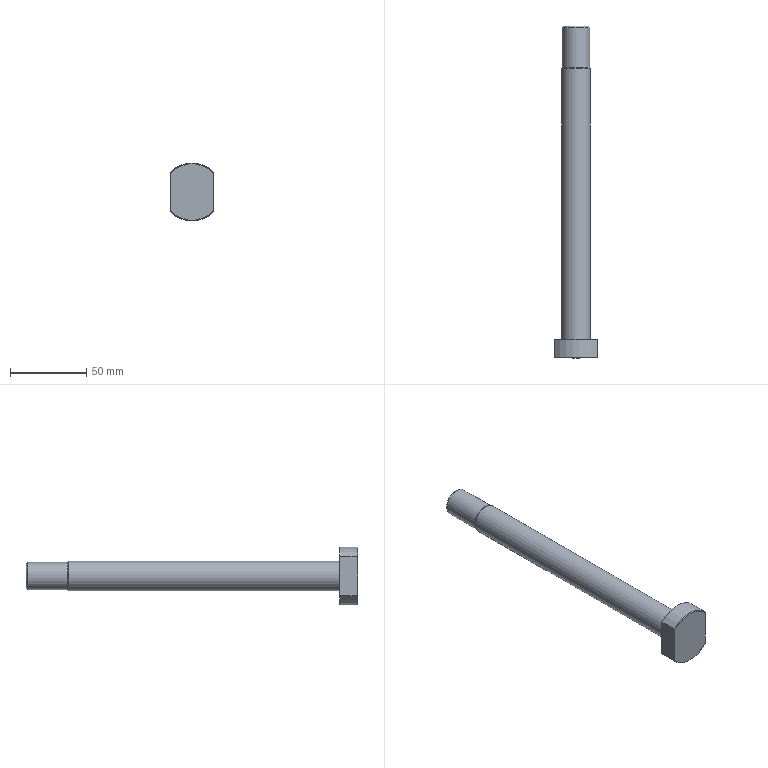Part | NX | features DATUM_CSYS 3, CHAMFER 2, SKETCH 2, BLEND 1, EXTRUDE 1, SWP104 1, SYMBOLIC_THREAD 1 | 1 solid | 13 faces | box 28 x 217 x 38 mm | volume 68775 mm3 | plane 5 | cylinder 4 | cone 3 | torus 1 | commonest cylinder face diameters 38 x2 18 x1 19 x1
STEP:
#1=CARTESIAN_POINT('',(-14.,-12.,-12.093));
#2=VERTEX_POINT('',#1);
#3=CARTESIAN_POINT('',(-14.,-12.,12.093));
#4=VERTEX_POINT('',#3);
#5=CARTESIAN_POINT('',(-14.,-12.,-19.));
#6=DIRECTION('',(0.,0.,1.));
#7=VECTOR('',#6,1000.);
#8=LINE('',#5,#7);
#9=EDGE_CURVE('',#2,#4,#8,.T.);
#10=ORIENTED_EDGE('',*,*,#9,.F.);
#11=CARTESIAN_POINT('',(14.,-12.,-12.093));
#12=VERTEX_POINT('',#11);
#13=CARTESIAN_POINT('',(0.,-12.,0.));
#14=DIRECTION('',(0.,1.,0.));
#15=DIRECTION('',(0.,0.,1.));
#16=AXIS2_PLACEMENT_3D('',#13,#14,#15);
#17=CIRCLE('',#16,18.5);
#18=EDGE_CURVE('',#2,#12,#17,.F.);
#19=ORIENTED_EDGE('',*,*,#18,.T.);
#20=CARTESIAN_POINT('',(14.,-12.,12.093));
#21=VERTEX_POINT('',#20);
#22=CARTESIAN_POINT('',(14.,-12.,19.));
#23=DIRECTION('',(0.,0.,-1.));
#24=VECTOR('',#23,1000.);
#25=LINE('',#22,#24);
#26=EDGE_CURVE('',#21,#12,#25,.T.);
#27=ORIENTED_EDGE('',*,*,#26,.F.);
#28=CARTESIAN_POINT('',(0.,-12.,0.));
#29=DIRECTION('',(0.,1.,0.));
#30=DIRECTION('',(0.,0.,1.));
#31=AXIS2_PLACEMENT_3D('',#28,#29,#30);
#32=CIRCLE('',#31,18.5);
#33=EDGE_CURVE('',#21,#4,#32,.F.);
#34=ORIENTED_EDGE('',*,*,#33,.T.);
#35=EDGE_LOOP('',(#10,#19,#27,#34));
#36=FACE_BOUND('',#35,.T.);
#37=CARTESIAN_POINT('',(0.,-12.,0.));
#38=DIRECTION('',(0.,1.,0.));
#39=DIRECTION('',(0.,0.,1.));
#40=AXIS2_PLACEMENT_3D('',#37,#38,#39);
#41=PLANE('',#40);
#42=ADVANCED_FACE('',(#36),#41,.F.);
#43=CARTESIAN_POINT('',(0.,0.,9.5));
#44=VERTEX_POINT('',#43);
#45=CARTESIAN_POINT('',(0.,0.,0.));
#46=DIRECTION('',(0.,1.,0.));
#47=DIRECTION('',(0.,0.,1.));
#48=AXIS2_PLACEMENT_3D('',#45,#46,#47);
#49=CIRCLE('',#48,9.5);
#50=EDGE_CURVE('',#44,#44,#49,.T.);
#51=ORIENTED_EDGE('',*,*,#50,.F.);
#52=EDGE_LOOP('',(#51));
#53=FACE_BOUND('',#52,.T.);
#54=CARTESIAN_POINT('',(14.,0.,-12.845));
#55=VERTEX_POINT('',#54);
#56=CARTESIAN_POINT('',(14.,0.,12.845));
#57=VERTEX_POINT('',#56);
#58=CARTESIAN_POINT('',(14.,0.,19.));
#59=DIRECTION('',(0.,0.,1.));
#60=VECTOR('',#59,1000.);
#61=LINE('',#58,#60);
#62=EDGE_CURVE('',#55,#57,#61,.T.);
#63=ORIENTED_EDGE('',*,*,#62,.F.);
#64=CARTESIAN_POINT('',(-14.,0.,-12.845));
#65=VERTEX_POINT('',#64);
#66=CARTESIAN_POINT('',(0.,0.,0.));
#67=DIRECTION('',(0.,1.,0.));
#68=DIRECTION('',(0.,0.,1.));
#69=AXIS2_PLACEMENT_3D('',#66,#67,#68);
#70=CIRCLE('',#69,19.);
#71=EDGE_CURVE('',#55,#65,#70,.T.);
#72=ORIENTED_EDGE('',*,*,#71,.T.);
#73=CARTESIAN_POINT('',(-14.,0.,12.845));
#74=VERTEX_POINT('',#73);
#75=CARTESIAN_POINT('',(-14.,0.,-19.));
#76=DIRECTION('',(0.,0.,-1.));
#77=VECTOR('',#76,1000.);
#78=LINE('',#75,#77);
#79=EDGE_CURVE('',#74,#65,#78,.T.);
#80=ORIENTED_EDGE('',*,*,#79,.F.);
#81=CARTESIAN_POINT('',(0.,0.,0.));
#82=DIRECTION('',(0.,1.,0.));
#83=DIRECTION('',(0.,0.,1.));
#84=AXIS2_PLACEMENT_3D('',#81,#82,#83);
#85=CIRCLE('',#84,19.);
#86=EDGE_CURVE('',#74,#57,#85,.T.);
#87=ORIENTED_EDGE('',*,*,#86,.T.);
#88=EDGE_LOOP('',(#63,#72,#80,#87));
#89=FACE_BOUND('',#88,.T.);
#90=CARTESIAN_POINT('',(0.,0.,19.));
#91=DIRECTION('',(0.,-1.,0.));
#92=DIRECTION('',(0.,0.,-1.));
#93=AXIS2_PLACEMENT_3D('',#90,#91,#92);
#94=PLANE('',#93);
#95=ADVANCED_FACE('',(#53,#89),#94,.F.);
#96=CARTESIAN_POINT('',(-14.,-11.5,12.845));
#97=VERTEX_POINT('',#96);
#98=CARTESIAN_POINT('',(-14.,0.,12.845));
#99=DIRECTION('',(0.,1.,0.));
#100=VECTOR('',#99,1000.);
#101=LINE('',#98,#100);
#102=EDGE_CURVE('',#97,#74,#101,.T.);
#103=ORIENTED_EDGE('',*,*,#102,.F.);
#104=CARTESIAN_POINT('',(14.,-11.5,12.845));
#105=VERTEX_POINT('',#104);
#106=CARTESIAN_POINT('',(0.,-11.5,0.));
#107=DIRECTION('',(0.,1.,0.));
#108=DIRECTION('',(0.,0.,1.));
#109=AXIS2_PLACEMENT_3D('',#106,#107,#108);
#110=CIRCLE('',#109,19.);
#111=EDGE_CURVE('',#97,#105,#110,.T.);
#112=ORIENTED_EDGE('',*,*,#111,.T.);
#113=CARTESIAN_POINT('',(14.,0.,12.845));
#114=DIRECTION('',(0.,1.,0.));
#115=VECTOR('',#114,1000.);
#116=LINE('',#113,#115);
#117=EDGE_CURVE('',#57,#105,#116,.F.);
#118=ORIENTED_EDGE('',*,*,#117,.F.);
#119=ORIENTED_EDGE('',*,*,#86,.F.);
#120=EDGE_LOOP('',(#103,#112,#118,#119));
#121=FACE_BOUND('',#120,.T.);
#122=CARTESIAN_POINT('',(0.,0.,0.));
#123=DIRECTION('',(0.,1.,0.));
#124=DIRECTION('',(0.,0.,1.));
#125=AXIS2_PLACEMENT_3D('',#122,#123,#124);
#126=CYLINDRICAL_SURFACE('',#125,19.);
#127=ADVANCED_FACE('',(#121),#126,.T.);
#128=CARTESIAN_POINT('',(14.,-11.5,-12.845));
#129=VERTEX_POINT('',#128);
#130=CARTESIAN_POINT('',(14.,0.,-12.845));
#131=DIRECTION('',(0.,1.,0.));
#132=VECTOR('',#131,1000.);
#133=LINE('',#130,#132);
#134=EDGE_CURVE('',#129,#55,#133,.T.);
#135=ORIENTED_EDGE('',*,*,#134,.F.);
#136=CARTESIAN_POINT('',(-14.,-11.5,-12.845));
#137=VERTEX_POINT('',#136);
#138=CARTESIAN_POINT('',(0.,-11.5,0.));
#139=DIRECTION('',(0.,1.,0.));
#140=DIRECTION('',(0.,0.,1.));
#141=AXIS2_PLACEMENT_3D('',#138,#139,#140);
#142=CIRCLE('',#141,19.);
#143=EDGE_CURVE('',#129,#137,#142,.T.);
#144=ORIENTED_EDGE('',*,*,#143,.T.);
#145=CARTESIAN_POINT('',(-14.,0.,-12.845));
#146=DIRECTION('',(0.,1.,0.));
#147=VECTOR('',#146,1000.);
#148=LINE('',#145,#147);
#149=EDGE_CURVE('',#65,#137,#148,.F.);
#150=ORIENTED_EDGE('',*,*,#149,.F.);
#151=ORIENTED_EDGE('',*,*,#71,.F.);
#152=EDGE_LOOP('',(#135,#144,#150,#151));
#153=FACE_BOUND('',#152,.T.);
#154=CARTESIAN_POINT('',(0.,0.,0.));
#155=DIRECTION('',(0.,1.,0.));
#156=DIRECTION('',(0.,0.,1.));
#157=AXIS2_PLACEMENT_3D('',#154,#155,#156);
#158=CYLINDRICAL_SURFACE('',#157,19.);
#159=ADVANCED_FACE('',(#153),#158,.T.);
#160=CARTESIAN_POINT('',(0.,205.,8.));
#161=VERTEX_POINT('',#160);
#162=CARTESIAN_POINT('',(0.,205.,0.));
#163=DIRECTION('',(0.,1.,0.));
#164=DIRECTION('',(0.,0.,1.));
#165=AXIS2_PLACEMENT_3D('',#162,#163,#164);
#166=CIRCLE('',#165,8.);
#167=EDGE_CURVE('',#161,#161,#166,.T.);
#168=ORIENTED_EDGE('',*,*,#167,.T.);
#169=EDGE_LOOP('',(#168));
#170=FACE_BOUND('',#169,.T.);
#171=CARTESIAN_POINT('',(0.,205.,0.));
#172=DIRECTION('',(0.,1.,0.));
#173=DIRECTION('',(0.,0.,1.));
#174=AXIS2_PLACEMENT_3D('',#171,#172,#173);
#175=PLANE('',#174);
#176=ADVANCED_FACE('',(#170),#175,.T.);
#177=CARTESIAN_POINT('',(0.,204.,9.));
#178=VERTEX_POINT('',#177);
#179=CARTESIAN_POINT('',(0.,204.,0.));
#180=DIRECTION('',(0.,1.,0.));
#181=DIRECTION('',(0.,0.,1.));
#182=AXIS2_PLACEMENT_3D('',#179,#180,#181);
#183=CIRCLE('',#182,9.);
#184=EDGE_CURVE('',#178,#178,#183,.F.);
#185=ORIENTED_EDGE('',*,*,#184,.T.);
#186=EDGE_LOOP('',(#185));
#187=FACE_BOUND('',#186,.T.);
#188=CARTESIAN_POINT('',(0.,177.866,-9.));
#189=VERTEX_POINT('',#188);
#190=CARTESIAN_POINT('',(0.,177.866,0.));
#191=DIRECTION('',(0.,-1.,0.));
#192=DIRECTION('',(0.,0.,-1.));
#193=AXIS2_PLACEMENT_3D('',#190,#191,#192);
#194=CIRCLE('',#193,9.);
#195=EDGE_CURVE('',#189,#189,#194,.F.);
#196=ORIENTED_EDGE('',*,*,#195,.T.);
#197=EDGE_LOOP('',(#196));
#198=FACE_BOUND('',#197,.T.);
#199=CARTESIAN_POINT('',(0.,0.,0.));
#200=DIRECTION('',(0.,1.,0.));
#201=DIRECTION('',(0.,0.,1.));
#202=AXIS2_PLACEMENT_3D('',#199,#200,#201);
#203=CYLINDRICAL_SURFACE('',#202,9.);
#204=ADVANCED_FACE('',(#187,#198),#203,.T.);
#205=CARTESIAN_POINT('',(0.,177.,9.5));
#206=VERTEX_POINT('',#205);
#207=CARTESIAN_POINT('',(0.,177.,0.));
#208=DIRECTION('',(0.,1.,0.));
#209=DIRECTION('',(0.,0.,1.));
#210=AXIS2_PLACEMENT_3D('',#207,#208,#209);
#211=CIRCLE('',#210,9.5);
#212=EDGE_CURVE('',#206,#206,#211,.T.);
#213=ORIENTED_EDGE('',*,*,#212,.F.);
#214=EDGE_LOOP('',(#213));
#215=FACE_BOUND('',#214,.T.);
#216=ORIENTED_EDGE('',*,*,#50,.T.);
#217=EDGE_LOOP('',(#216));
#218=FACE_BOUND('',#217,.T.);
#219=CARTESIAN_POINT('',(0.,0.,0.));
#220=DIRECTION('',(0.,1.,0.));
#221=DIRECTION('',(0.,0.,1.));
#222=AXIS2_PLACEMENT_3D('',#219,#220,#221);
#223=CYLINDRICAL_SURFACE('',#222,9.5);
#224=ADVANCED_FACE('',(#215,#218),#223,.T.);
#225=ORIENTED_EDGE('',*,*,#212,.T.);
#226=EDGE_LOOP('',(#225));
#227=FACE_BOUND('',#226,.T.);
#228=ORIENTED_EDGE('',*,*,#195,.F.);
#229=EDGE_LOOP('',(#228));
#230=FACE_BOUND('',#229,.T.);
#231=CARTESIAN_POINT('',(0.,177.866,0.));
#232=DIRECTION('',(0.,-1.,0.));
#233=DIRECTION('',(0.,0.,-1.));
#234=AXIS2_PLACEMENT_3D('',#231,#232,#233);
#235=TOROIDAL_SURFACE('',#234,10.,1.);
#236=ADVANCED_FACE('',(#227,#230),#235,.F.);
#237=ORIENTED_EDGE('',*,*,#149,.T.);
#238=CARTESIAN_POINT('',(-14.,-11.5,-12.845));
#239=CARTESIAN_POINT('',(-14.,-11.669,-12.596));
#240=CARTESIAN_POINT('',(-14.,-11.835,-12.345));
#241=CARTESIAN_POINT('',(-14.,-12.,-12.093));
#242=B_SPLINE_CURVE_WITH_KNOTS('',3,(#238,#239,#240,#241),.UNSPECIFIED.,.F.,.F.,(4,4),(0.,0.0009029),.UNSPECIFIED.);
#243=EDGE_CURVE('',#137,#2,#242,.T.);
#244=ORIENTED_EDGE('',*,*,#243,.T.);
#245=ORIENTED_EDGE('',*,*,#9,.T.);
#246=CARTESIAN_POINT('',(-14.,-12.,12.093));
#247=CARTESIAN_POINT('',(-14.,-11.835,12.345));
#248=CARTESIAN_POINT('',(-14.,-11.669,12.596));
#249=CARTESIAN_POINT('',(-14.,-11.5,12.845));
#250=B_SPLINE_CURVE_WITH_KNOTS('',3,(#246,#247,#248,#249),.UNSPECIFIED.,.F.,.F.,(4,4),(0.,0.0009029),.UNSPECIFIED.);
#251=EDGE_CURVE('',#4,#97,#250,.T.);
#252=ORIENTED_EDGE('',*,*,#251,.T.);
#253=ORIENTED_EDGE('',*,*,#102,.T.);
#254=ORIENTED_EDGE('',*,*,#79,.T.);
#255=EDGE_LOOP('',(#237,#244,#245,#252,#253,#254));
#256=FACE_BOUND('',#255,.T.);
#257=CARTESIAN_POINT('',(-14.,106.8,-19.));
#258=DIRECTION('',(1.,0.,0.));
#259=DIRECTION('',(0.,0.,-1.));
#260=AXIS2_PLACEMENT_3D('',#257,#258,#259);
#261=PLANE('',#260);
#262=ADVANCED_FACE('',(#256),#261,.F.);
#263=ORIENTED_EDGE('',*,*,#26,.T.);
#264=CARTESIAN_POINT('',(14.,-12.,-12.093));
#265=CARTESIAN_POINT('',(14.,-11.835,-12.345));
#266=CARTESIAN_POINT('',(14.,-11.669,-12.596));
#267=CARTESIAN_POINT('',(14.,-11.5,-12.845));
#268=B_SPLINE_CURVE_WITH_KNOTS('',3,(#264,#265,#266,#267),.UNSPECIFIED.,.F.,.F.,(4,4),(0.,0.0009029),.UNSPECIFIED.);
#269=EDGE_CURVE('',#12,#129,#268,.T.);
#270=ORIENTED_EDGE('',*,*,#269,.T.);
#271=ORIENTED_EDGE('',*,*,#134,.T.);
#272=ORIENTED_EDGE('',*,*,#62,.T.);
#273=ORIENTED_EDGE('',*,*,#117,.T.);
#274=CARTESIAN_POINT('',(14.,-11.5,12.845));
#275=CARTESIAN_POINT('',(14.,-11.669,12.596));
#276=CARTESIAN_POINT('',(14.,-11.835,12.345));
#277=CARTESIAN_POINT('',(14.,-12.,12.093));
#278=B_SPLINE_CURVE_WITH_KNOTS('',3,(#274,#275,#276,#277),.UNSPECIFIED.,.F.,.F.,(4,4),(0.,0.0009029),.UNSPECIFIED.);
#279=EDGE_CURVE('',#105,#21,#278,.T.);
#280=ORIENTED_EDGE('',*,*,#279,.T.);
#281=EDGE_LOOP('',(#263,#270,#271,#272,#273,#280));
#282=FACE_BOUND('',#281,.T.);
#283=CARTESIAN_POINT('',(14.,106.8,19.));
#284=DIRECTION('',(-1.,0.,0.));
#285=DIRECTION('',(0.,0.,1.));
#286=AXIS2_PLACEMENT_3D('',#283,#284,#285);
#287=PLANE('',#286);
#288=ADVANCED_FACE('',(#282),#287,.F.);
#289=ORIENTED_EDGE('',*,*,#184,.F.);
#290=EDGE_LOOP('',(#289));
#291=FACE_BOUND('',#290,.T.);
#292=ORIENTED_EDGE('',*,*,#167,.F.);
#293=EDGE_LOOP('',(#292));
#294=FACE_BOUND('',#293,.T.);
#295=CARTESIAN_POINT('',(0.,205.,0.));
#296=DIRECTION('',(0.,-1.,0.));
#297=DIRECTION('',(0.,0.,-1.));
#298=AXIS2_PLACEMENT_3D('',#295,#296,#297);
#299=CONICAL_SURFACE('',#298,8.,0.7854);
#300=ADVANCED_FACE('',(#291,#294),#299,.T.);
#301=ORIENTED_EDGE('',*,*,#269,.F.);
#302=ORIENTED_EDGE('',*,*,#18,.F.);
#303=ORIENTED_EDGE('',*,*,#243,.F.);
#304=ORIENTED_EDGE('',*,*,#143,.F.);
#305=EDGE_LOOP('',(#301,#302,#303,#304));
#306=FACE_BOUND('',#305,.T.);
#307=CARTESIAN_POINT('',(0.,-11.5,0.));
#308=DIRECTION('',(0.,1.,0.));
#309=DIRECTION('',(0.,0.,1.));
#310=AXIS2_PLACEMENT_3D('',#307,#308,#309);
#311=CONICAL_SURFACE('',#310,19.,0.7854);
#312=ADVANCED_FACE('',(#306),#311,.T.);
#313=ORIENTED_EDGE('',*,*,#251,.F.);
#314=ORIENTED_EDGE('',*,*,#33,.F.);
#315=ORIENTED_EDGE('',*,*,#279,.F.);
#316=ORIENTED_EDGE('',*,*,#111,.F.);
#317=EDGE_LOOP('',(#313,#314,#315,#316));
#318=FACE_BOUND('',#317,.T.);
#319=CARTESIAN_POINT('',(0.,-11.5,0.));
#320=DIRECTION('',(0.,1.,0.));
#321=DIRECTION('',(0.,0.,1.));
#322=AXIS2_PLACEMENT_3D('',#319,#320,#321);
#323=CONICAL_SURFACE('',#322,19.,0.7854);
#324=ADVANCED_FACE('',(#318),#323,.T.);
#325=CLOSED_SHELL('',(#42,#95,#127,#159,#176,#204,#224,#236,#262,#288,#300,#312,#324));
#326=MANIFOLD_SOLID_BREP('',#325);
#327=(LENGTH_UNIT()NAMED_UNIT(*)SI_UNIT(.MILLI.,.METRE.));
#328=UNCERTAINTY_MEASURE_WITH_UNIT(LENGTH_MEASURE(0.0508),#327,'','');
#329=(NAMED_UNIT(*)PLANE_ANGLE_UNIT()SI_UNIT($,.RADIAN.));
#330=(NAMED_UNIT(*)SI_UNIT($,.STERADIAN.)SOLID_ANGLE_UNIT());
#331=(GEOMETRIC_REPRESENTATION_CONTEXT(3)GLOBAL_UNCERTAINTY_ASSIGNED_CONTEXT((#328))GLOBAL_UNIT_ASSIGNED_CONTEXT((#327,#329,#330))REPRESENTATION_CONTEXT('',''));
#332=ADVANCED_BREP_SHAPE_REPRESENTATION('',(#326),#331);